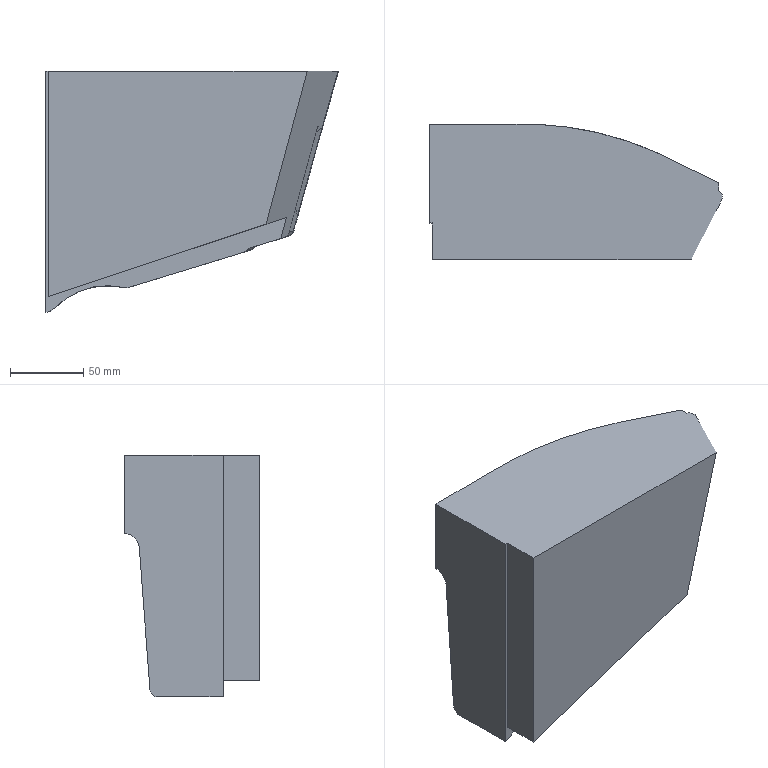Part | NX | features solid 2 | 1 solid | 70 faces | box 200.404 x 92.687 x 165.259 mm | volume 1812939 mm3 | spline 56 | plane 12 | cylinder 1 | sphere 1 | commonest cylinder face diameters 10 x1